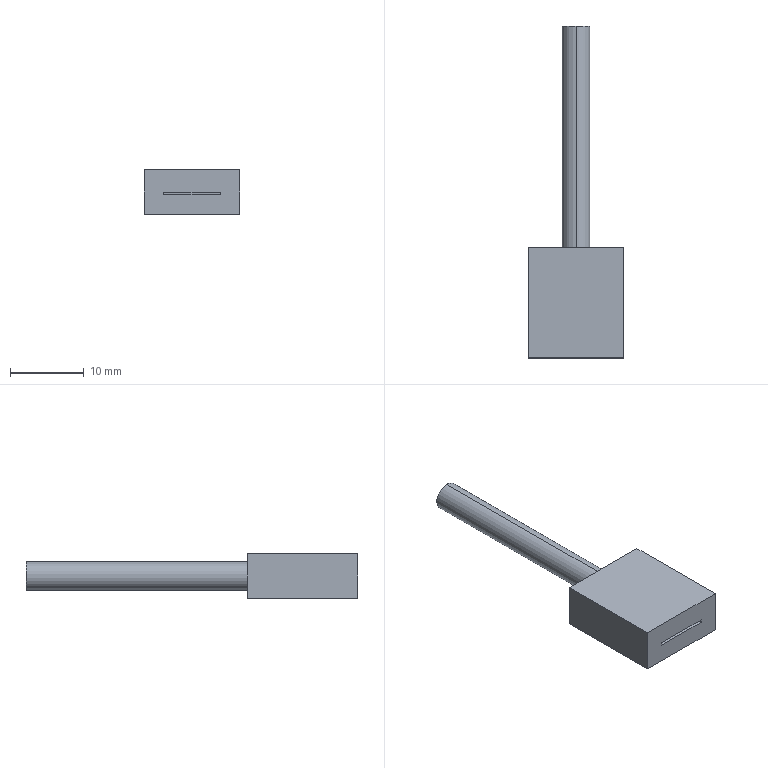Part | STEP file | 0244_012_FPCN14H | 1 solid | 14 faces | box 13 x 45 x 6 mm | volume 1495 mm3 | plane 12 | cylinder 2 | commonest cylinder face diameters 3.8 x2
STEP:
#1=CARTESIAN_POINT('',(0.,0.,0.));
#2=DIRECTION('',(0.,0.,1.));
#3=DIRECTION('',(1.,0.,0.));
#4=AXIS2_PLACEMENT_3D('',#1,#2,#3);
#5=CARTESIAN_POINT('',(0.,45.,-4.9));
#6=VERTEX_POINT('',#5);
#7=CARTESIAN_POINT('',(0.,45.,-1.1));
#8=VERTEX_POINT('',#7);
#9=CARTESIAN_POINT('',(0.,45.,-3.));
#10=DIRECTION('',(0.,-1.,0.));
#11=DIRECTION('',(0.,0.,-1.));
#12=AXIS2_PLACEMENT_3D('',#9,#10,#11);
#13=CIRCLE('',#12,1.9);
#14=CARTESIAN_POINT('',(0.,45.,-3.));
#15=DIRECTION('',(0.,-1.,0.));
#16=DIRECTION('',(0.,0.,-1.));
#17=AXIS2_PLACEMENT_3D('',#14,#15,#16);
#18=CYLINDRICAL_SURFACE('',#17,1.9);
#19=CARTESIAN_POINT('',(0.,0.));
#20=DIRECTION('',(1.,0.));
#21=VECTOR('',#20,1.);
#22=LINE('',#19,#21);
#23=(GEOMETRIC_REPRESENTATION_CONTEXT(2)PARAMETRIC_REPRESENTATION_CONTEXT()REPRESENTATION_CONTEXT('',''));
#24=DEFINITIONAL_REPRESENTATION('',(#22),#23);
#25=PCURVE('',#18,#24);
#26=CARTESIAN_POINT('',(0.,45.,-3.));
#27=DIRECTION('',(0.,1.,0.));
#28=DIRECTION('',(0.,0.,1.));
#29=AXIS2_PLACEMENT_3D('',#26,#27,#28);
#30=PLANE('',#29);
#31=CARTESIAN_POINT('',(-1.9,0.));
#32=CARTESIAN_POINT('',(-1.9,3.291));
#33=CARTESIAN_POINT('',(0.95,1.645));
#34=CARTESIAN_POINT('',(3.8,0.));
#35=CARTESIAN_POINT('',(0.95,-1.645));
#36=CARTESIAN_POINT('',(-1.9,-3.291));
#37=CARTESIAN_POINT('',(-1.9,0.));
#38=(BOUNDED_CURVE()B_SPLINE_CURVE(2,(#31,#32,#33,#34,#35,#36,#37),.UNSPECIFIED.,.T.,.F.)B_SPLINE_CURVE_WITH_KNOTS((1,2,2,2,2,1),(-2.094,0.,2.094,4.189,6.283,8.378),.UNSPECIFIED.)CURVE()GEOMETRIC_REPRESENTATION_ITEM()RATIONAL_B_SPLINE_CURVE((1.,0.5,1.,0.5,1.,0.5,1.))REPRESENTATION_ITEM(''));
#39=(GEOMETRIC_REPRESENTATION_CONTEXT(2)PARAMETRIC_REPRESENTATION_CONTEXT()REPRESENTATION_CONTEXT('',''));
#40=DEFINITIONAL_REPRESENTATION('',(#38),#39);
#41=PCURVE('',#30,#40);
#42=SURFACE_CURVE('',#13,(#25,#41),.PCURVE_S1.);
#43=EDGE_CURVE('',#6,#8,#42,.T.);
#44=ORIENTED_EDGE('',*,*,#43,.T.);
#45=CARTESIAN_POINT('',(0.,15.,-1.1));
#46=VERTEX_POINT('',#45);
#47=CARTESIAN_POINT('',(0.,45.,-1.1));
#48=DIRECTION('',(0.,-1.,0.));
#49=VECTOR('',#48,1.);
#50=LINE('',#47,#49);
#51=CARTESIAN_POINT('',(3.142,0.));
#52=DIRECTION('',(0.,1.));
#53=VECTOR('',#52,1.);
#54=LINE('',#51,#53);
#55=(GEOMETRIC_REPRESENTATION_CONTEXT(2)PARAMETRIC_REPRESENTATION_CONTEXT()REPRESENTATION_CONTEXT('',''));
#56=DEFINITIONAL_REPRESENTATION('',(#54),#55);
#57=PCURVE('',#18,#56);
#58=CARTESIAN_POINT('',(0.,45.,-3.));
#59=DIRECTION('',(0.,-1.,0.));
#60=DIRECTION('',(0.,0.,-1.));
#61=AXIS2_PLACEMENT_3D('',#58,#59,#60);
#62=CYLINDRICAL_SURFACE('',#61,1.9);
#63=CARTESIAN_POINT('',(3.142,0.));
#64=DIRECTION('',(0.,1.));
#65=VECTOR('',#64,1.);
#66=LINE('',#63,#65);
#67=(GEOMETRIC_REPRESENTATION_CONTEXT(2)PARAMETRIC_REPRESENTATION_CONTEXT()REPRESENTATION_CONTEXT('',''));
#68=DEFINITIONAL_REPRESENTATION('',(#66),#67);
#69=PCURVE('',#62,#68);
#70=SURFACE_CURVE('',#50,(#57,#69),.PCURVE_S1.);
#71=EDGE_CURVE('',#8,#46,#70,.T.);
#72=ORIENTED_EDGE('',*,*,#71,.T.);
#73=CARTESIAN_POINT('',(0.,15.,-4.9));
#74=VERTEX_POINT('',#73);
#75=CARTESIAN_POINT('',(0.,15.,-3.));
#76=DIRECTION('',(0.,1.,0.));
#77=DIRECTION('',(0.,0.,-1.));
#78=AXIS2_PLACEMENT_3D('',#75,#76,#77);
#79=CIRCLE('',#78,1.9);
#80=CARTESIAN_POINT('',(6.283,30.));
#81=DIRECTION('',(-1.,0.));
#82=VECTOR('',#81,1.);
#83=LINE('',#80,#82);
#84=(GEOMETRIC_REPRESENTATION_CONTEXT(2)PARAMETRIC_REPRESENTATION_CONTEXT()REPRESENTATION_CONTEXT('',''));
#85=DEFINITIONAL_REPRESENTATION('',(#83),#84);
#86=PCURVE('',#18,#85);
#87=CARTESIAN_POINT('',(6.5,15.,0.));
#88=DIRECTION('',(0.,-1.,0.));
#89=DIRECTION('',(0.,0.,-1.));
#90=AXIS2_PLACEMENT_3D('',#87,#88,#89);
#91=PLANE('',#90);
#92=CARTESIAN_POINT('',(4.9,-6.5));
#93=CARTESIAN_POINT('',(4.9,-9.791));
#94=CARTESIAN_POINT('',(2.05,-8.145));
#95=CARTESIAN_POINT('',(-0.8,-6.5));
#96=CARTESIAN_POINT('',(2.05,-4.855));
#97=CARTESIAN_POINT('',(4.9,-3.209));
#98=CARTESIAN_POINT('',(4.9,-6.5));
#99=(BOUNDED_CURVE()B_SPLINE_CURVE(2,(#92,#93,#94,#95,#96,#97,#98),.UNSPECIFIED.,.T.,.F.)B_SPLINE_CURVE_WITH_KNOTS((1,2,2,2,2,1),(-2.094,0.,2.094,4.189,6.283,8.378),.UNSPECIFIED.)CURVE()GEOMETRIC_REPRESENTATION_ITEM()RATIONAL_B_SPLINE_CURVE((1.,0.5,1.,0.5,1.,0.5,1.))REPRESENTATION_ITEM(''));
#100=(GEOMETRIC_REPRESENTATION_CONTEXT(2)PARAMETRIC_REPRESENTATION_CONTEXT()REPRESENTATION_CONTEXT('',''));
#101=DEFINITIONAL_REPRESENTATION('',(#99),#100);
#102=PCURVE('',#91,#101);
#103=SURFACE_CURVE('',#79,(#86,#102),.PCURVE_S1.);
#104=EDGE_CURVE('',#46,#74,#103,.T.);
#105=ORIENTED_EDGE('',*,*,#104,.T.);
#106=CARTESIAN_POINT('',(0.,45.,-4.9));
#107=DIRECTION('',(0.,-1.,0.));
#108=VECTOR('',#107,1.);
#109=LINE('',#106,#108);
#110=CARTESIAN_POINT('',(0.,0.));
#111=DIRECTION('',(0.,1.));
#112=VECTOR('',#111,1.);
#113=LINE('',#110,#112);
#114=(GEOMETRIC_REPRESENTATION_CONTEXT(2)PARAMETRIC_REPRESENTATION_CONTEXT()REPRESENTATION_CONTEXT('',''));
#115=DEFINITIONAL_REPRESENTATION('',(#113),#114);
#116=PCURVE('',#18,#115);
#117=CARTESIAN_POINT('',(6.283,0.));
#118=DIRECTION('',(0.,1.));
#119=VECTOR('',#118,1.);
#120=LINE('',#117,#119);
#121=(GEOMETRIC_REPRESENTATION_CONTEXT(2)PARAMETRIC_REPRESENTATION_CONTEXT()REPRESENTATION_CONTEXT('',''));
#122=DEFINITIONAL_REPRESENTATION('',(#120),#121);
#123=PCURVE('',#62,#122);
#124=SURFACE_CURVE('',#109,(#116,#123),.PCURVE_S1.);
#125=EDGE_CURVE('',#6,#74,#124,.T.);
#126=ORIENTED_EDGE('',*,*,#125,.F.);
#127=EDGE_LOOP('',(#44,#72,#105,#126));
#128=FACE_BOUND('',#127,.T.);
#129=ADVANCED_FACE('',(#128),#18,.T.);
#130=CARTESIAN_POINT('',(6.5,0.,0.));
#131=VERTEX_POINT('',#130);
#132=CARTESIAN_POINT('',(-6.5,0.,0.));
#133=VERTEX_POINT('',#132);
#134=CARTESIAN_POINT('',(6.5,0.,0.));
#135=DIRECTION('',(-1.,0.,0.));
#136=VECTOR('',#135,1.);
#137=LINE('',#134,#136);
#138=CARTESIAN_POINT('',(6.5,0.,0.));
#139=DIRECTION('',(0.,0.,-1.));
#140=DIRECTION('',(-1.,0.,0.));
#141=AXIS2_PLACEMENT_3D('',#138,#139,#140);
#142=PLANE('',#141);
#143=CARTESIAN_POINT('',(0.,0.));
#144=DIRECTION('',(1.,0.));
#145=VECTOR('',#144,1.);
#146=LINE('',#143,#145);
#147=(GEOMETRIC_REPRESENTATION_CONTEXT(2)PARAMETRIC_REPRESENTATION_CONTEXT()REPRESENTATION_CONTEXT('',''));
#148=DEFINITIONAL_REPRESENTATION('',(#146),#147);
#149=PCURVE('',#142,#148);
#150=CARTESIAN_POINT('',(6.5,0.,0.));
#151=DIRECTION('',(0.,1.,0.));
#152=DIRECTION('',(0.,0.,1.));
#153=AXIS2_PLACEMENT_3D('',#150,#151,#152);
#154=PLANE('',#153);
#155=CARTESIAN_POINT('',(0.,0.));
#156=DIRECTION('',(0.,-1.));
#157=VECTOR('',#156,1.);
#158=LINE('',#155,#157);
#159=(GEOMETRIC_REPRESENTATION_CONTEXT(2)PARAMETRIC_REPRESENTATION_CONTEXT()REPRESENTATION_CONTEXT('',''));
#160=DEFINITIONAL_REPRESENTATION('',(#158),#159);
#161=PCURVE('',#154,#160);
#162=SURFACE_CURVE('',#137,(#149,#161),.PCURVE_S1.);
#163=EDGE_CURVE('',#131,#133,#162,.T.);
#164=ORIENTED_EDGE('',*,*,#163,.F.);
#165=CARTESIAN_POINT('',(6.5,15.,0.));
#166=VERTEX_POINT('',#165);
#167=CARTESIAN_POINT('',(6.5,0.,0.));
#168=DIRECTION('',(0.,-1.,0.));
#169=VECTOR('',#168,1.);
#170=LINE('',#167,#169);
#171=CARTESIAN_POINT('',(0.,0.));
#172=DIRECTION('',(0.,-1.));
#173=VECTOR('',#172,1.);
#174=LINE('',#171,#173);
#175=(GEOMETRIC_REPRESENTATION_CONTEXT(2)PARAMETRIC_REPRESENTATION_CONTEXT()REPRESENTATION_CONTEXT('',''));
#176=DEFINITIONAL_REPRESENTATION('',(#174),#175);
#177=PCURVE('',#142,#176);
#178=CARTESIAN_POINT('',(6.5,15.,0.));
#179=DIRECTION('',(-1.,0.,0.));
#180=DIRECTION('',(0.,0.,1.));
#181=AXIS2_PLACEMENT_3D('',#178,#179,#180);
#182=PLANE('',#181);
#183=CARTESIAN_POINT('',(0.,-15.));
#184=DIRECTION('',(0.,-1.));
#185=VECTOR('',#184,1.);
#186=LINE('',#183,#185);
#187=(GEOMETRIC_REPRESENTATION_CONTEXT(2)PARAMETRIC_REPRESENTATION_CONTEXT()REPRESENTATION_CONTEXT('',''));
#188=DEFINITIONAL_REPRESENTATION('',(#186),#187);
#189=PCURVE('',#182,#188);
#190=SURFACE_CURVE('',#170,(#177,#189),.PCURVE_S1.);
#191=EDGE_CURVE('',#166,#131,#190,.T.);
#192=ORIENTED_EDGE('',*,*,#191,.F.);
#193=CARTESIAN_POINT('',(-6.5,15.,0.));
#194=VERTEX_POINT('',#193);
#195=CARTESIAN_POINT('',(6.5,15.,0.));
#196=DIRECTION('',(1.,0.,0.));
#197=VECTOR('',#196,1.);
#198=LINE('',#195,#197);
#199=CARTESIAN_POINT('',(0.,15.));
#200=DIRECTION('',(-1.,0.));
#201=VECTOR('',#200,1.);
#202=LINE('',#199,#201);
#203=(GEOMETRIC_REPRESENTATION_CONTEXT(2)PARAMETRIC_REPRESENTATION_CONTEXT()REPRESENTATION_CONTEXT('',''));
#204=DEFINITIONAL_REPRESENTATION('',(#202),#203);
#205=PCURVE('',#142,#204);
#206=CARTESIAN_POINT('',(0.,0.));
#207=DIRECTION('',(0.,1.));
#208=VECTOR('',#207,1.);
#209=LINE('',#206,#208);
#210=(GEOMETRIC_REPRESENTATION_CONTEXT(2)PARAMETRIC_REPRESENTATION_CONTEXT()REPRESENTATION_CONTEXT('',''));
#211=DEFINITIONAL_REPRESENTATION('',(#209),#210);
#212=PCURVE('',#91,#211);
#213=SURFACE_CURVE('',#198,(#205,#212),.PCURVE_S1.);
#214=EDGE_CURVE('',#194,#166,#213,.T.);
#215=ORIENTED_EDGE('',*,*,#214,.F.);
#216=CARTESIAN_POINT('',(-6.5,0.,0.));
#217=DIRECTION('',(0.,1.,0.));
#218=VECTOR('',#217,1.);
#219=LINE('',#216,#218);
#220=CARTESIAN_POINT('',(13.,0.));
#221=DIRECTION('',(0.,1.));
#222=VECTOR('',#221,1.);
#223=LINE('',#220,#222);
#224=(GEOMETRIC_REPRESENTATION_CONTEXT(2)PARAMETRIC_REPRESENTATION_CONTEXT()REPRESENTATION_CONTEXT('',''));
#225=DEFINITIONAL_REPRESENTATION('',(#223),#224);
#226=PCURVE('',#142,#225);
#227=CARTESIAN_POINT('',(-6.5,15.,0.));
#228=DIRECTION('',(-1.,0.,0.));
#229=DIRECTION('',(0.,0.,1.));
#230=AXIS2_PLACEMENT_3D('',#227,#228,#229);
#231=PLANE('',#230);
#232=CARTESIAN_POINT('',(0.,-15.));
#233=DIRECTION('',(0.,1.));
#234=VECTOR('',#233,1.);
#235=LINE('',#232,#234);
#236=(GEOMETRIC_REPRESENTATION_CONTEXT(2)PARAMETRIC_REPRESENTATION_CONTEXT()REPRESENTATION_CONTEXT('',''));
#237=DEFINITIONAL_REPRESENTATION('',(#235),#236);
#238=PCURVE('',#231,#237);
#239=SURFACE_CURVE('',#219,(#226,#238),.PCURVE_S1.);
#240=EDGE_CURVE('',#133,#194,#239,.T.);
#241=ORIENTED_EDGE('',*,*,#240,.F.);
#242=EDGE_LOOP('',(#164,#192,#215,#241));
#243=FACE_BOUND('',#242,.T.);
#244=ADVANCED_FACE('',(#243),#142,.F.);
#245=CARTESIAN_POINT('',(-6.5,15.,-6.));
#246=VERTEX_POINT('',#245);
#247=CARTESIAN_POINT('',(-6.5,0.,-6.));
#248=VERTEX_POINT('',#247);
#249=CARTESIAN_POINT('',(-6.5,15.,-6.));
#250=DIRECTION('',(0.,-1.,0.));
#251=VECTOR('',#250,1.);
#252=LINE('',#249,#251);
#253=CARTESIAN_POINT('',(-6.,0.));
#254=DIRECTION('',(0.,-1.));
#255=VECTOR('',#254,1.);
#256=LINE('',#253,#255);
#257=(GEOMETRIC_REPRESENTATION_CONTEXT(2)PARAMETRIC_REPRESENTATION_CONTEXT()REPRESENTATION_CONTEXT('',''));
#258=DEFINITIONAL_REPRESENTATION('',(#256),#257);
#259=PCURVE('',#231,#258);
#260=CARTESIAN_POINT('',(6.5,0.,-6.));
#261=DIRECTION('',(0.,0.,1.));
#262=DIRECTION('',(1.,0.,0.));
#263=AXIS2_PLACEMENT_3D('',#260,#261,#262);
#264=PLANE('',#263);
#265=CARTESIAN_POINT('',(-13.,15.));
#266=DIRECTION('',(0.,-1.));
#267=VECTOR('',#266,1.);
#268=LINE('',#265,#267);
#269=(GEOMETRIC_REPRESENTATION_CONTEXT(2)PARAMETRIC_REPRESENTATION_CONTEXT()REPRESENTATION_CONTEXT('',''));
#270=DEFINITIONAL_REPRESENTATION('',(#268),#269);
#271=PCURVE('',#264,#270);
#272=SURFACE_CURVE('',#252,(#259,#271),.PCURVE_S1.);
#273=EDGE_CURVE('',#246,#248,#272,.T.);
#274=ORIENTED_EDGE('',*,*,#273,.T.);
#275=CARTESIAN_POINT('',(-6.5,0.,0.));
#276=DIRECTION('',(0.,0.,1.));
#277=VECTOR('',#276,1.);
#278=LINE('',#275,#277);
#279=CARTESIAN_POINT('',(0.,-15.));
#280=DIRECTION('',(1.,0.));
#281=VECTOR('',#280,1.);
#282=LINE('',#279,#281);
#283=(GEOMETRIC_REPRESENTATION_CONTEXT(2)PARAMETRIC_REPRESENTATION_CONTEXT()REPRESENTATION_CONTEXT('',''));
#284=DEFINITIONAL_REPRESENTATION('',(#282),#283);
#285=PCURVE('',#231,#284);
#286=CARTESIAN_POINT('',(0.,-13.));
#287=DIRECTION('',(1.,0.));
#288=VECTOR('',#287,1.);
#289=LINE('',#286,#288);
#290=(GEOMETRIC_REPRESENTATION_CONTEXT(2)PARAMETRIC_REPRESENTATION_CONTEXT()REPRESENTATION_CONTEXT('',''));
#291=DEFINITIONAL_REPRESENTATION('',(#289),#290);
#292=PCURVE('',#154,#291);
#293=SURFACE_CURVE('',#278,(#285,#292),.PCURVE_S1.);
#294=EDGE_CURVE('',#248,#133,#293,.T.);
#295=ORIENTED_EDGE('',*,*,#294,.T.);
#296=ORIENTED_EDGE('',*,*,#240,.T.);
#297=CARTESIAN_POINT('',(-6.5,15.,0.));
#298=DIRECTION('',(0.,0.,-1.));
#299=VECTOR('',#298,1.);
#300=LINE('',#297,#299);
#301=CARTESIAN_POINT('',(0.,0.));
#302=DIRECTION('',(-1.,0.));
#303=VECTOR('',#302,1.);
#304=LINE('',#301,#303);
#305=(GEOMETRIC_REPRESENTATION_CONTEXT(2)PARAMETRIC_REPRESENTATION_CONTEXT()REPRESENTATION_CONTEXT('',''));
#306=DEFINITIONAL_REPRESENTATION('',(#304),#305);
#307=PCURVE('',#231,#306);
#308=CARTESIAN_POINT('',(0.,-13.));
#309=DIRECTION('',(1.,0.));
#310=VECTOR('',#309,1.);
#311=LINE('',#308,#310);
#312=(GEOMETRIC_REPRESENTATION_CONTEXT(2)PARAMETRIC_REPRESENTATION_CONTEXT()REPRESENTATION_CONTEXT('',''));
#313=DEFINITIONAL_REPRESENTATION('',(#311),#312);
#314=PCURVE('',#91,#313);
#315=SURFACE_CURVE('',#300,(#307,#314),.PCURVE_S1.);
#316=EDGE_CURVE('',#194,#246,#315,.T.);
#317=ORIENTED_EDGE('',*,*,#316,.T.);
#318=EDGE_LOOP('',(#274,#295,#296,#317));
#319=FACE_BOUND('',#318,.T.);
#320=ADVANCED_FACE('',(#319),#231,.T.);
#321=CARTESIAN_POINT('',(6.5,0.,-6.));
#322=VERTEX_POINT('',#321);
#323=CARTESIAN_POINT('',(6.5,0.,-6.));
#324=DIRECTION('',(-1.,0.,0.));
#325=VECTOR('',#324,1.);
#326=LINE('',#323,#325);
#327=CARTESIAN_POINT('',(-6.,0.));
#328=DIRECTION('',(0.,-1.));
#329=VECTOR('',#328,1.);
#330=LINE('',#327,#329);
#331=(GEOMETRIC_REPRESENTATION_CONTEXT(2)PARAMETRIC_REPRESENTATION_CONTEXT()REPRESENTATION_CONTEXT('',''));
#332=DEFINITIONAL_REPRESENTATION('',(#330),#331);
#333=PCURVE('',#154,#332);
#334=CARTESIAN_POINT('',(0.,0.));
#335=DIRECTION('',(-1.,0.));
#336=VECTOR('',#335,1.);
#337=LINE('',#334,#336);
#338=(GEOMETRIC_REPRESENTATION_CONTEXT(2)PARAMETRIC_REPRESENTATION_CONTEXT()REPRESENTATION_CONTEXT('',''));
#339=DEFINITIONAL_REPRESENTATION('',(#337),#338);
#340=PCURVE('',#264,#339);
#341=SURFACE_CURVE('',#326,(#333,#340),.PCURVE_S1.);
#342=EDGE_CURVE('',#322,#248,#341,.T.);
#343=ORIENTED_EDGE('',*,*,#342,.F.);
#344=CARTESIAN_POINT('',(6.5,0.,0.));
#345=DIRECTION('',(0.,0.,-1.));
#346=VECTOR('',#345,1.);
#347=LINE('',#344,#346);
#348=CARTESIAN_POINT('',(0.,0.));
#349=DIRECTION('',(-1.,0.));
#350=VECTOR('',#349,1.);
#351=LINE('',#348,#350);
#352=(GEOMETRIC_REPRESENTATION_CONTEXT(2)PARAMETRIC_REPRESENTATION_CONTEXT()REPRESENTATION_CONTEXT('',''));
#353=DEFINITIONAL_REPRESENTATION('',(#351),#352);
#354=PCURVE('',#154,#353);
#355=CARTESIAN_POINT('',(0.,-15.));
#356=DIRECTION('',(-1.,0.));
#357=VECTOR('',#356,1.);
#358=LINE('',#355,#357);
#359=(GEOMETRIC_REPRESENTATION_CONTEXT(2)PARAMETRIC_REPRESENTATION_CONTEXT()REPRESENTATION_CONTEXT('',''));
#360=DEFINITIONAL_REPRESENTATION('',(#358),#359);
#361=PCURVE('',#182,#360);
#362=SURFACE_CURVE('',#347,(#354,#361),.PCURVE_S1.);
#363=EDGE_CURVE('',#131,#322,#362,.T.);
#364=ORIENTED_EDGE('',*,*,#363,.F.);
#365=ORIENTED_EDGE('',*,*,#163,.T.);
#366=ORIENTED_EDGE('',*,*,#294,.F.);
#367=EDGE_LOOP('',(#343,#364,#365,#366));
#368=FACE_BOUND('',#367,.T.);
#369=CARTESIAN_POINT('',(-3.8,0.,-3.4));
#370=VERTEX_POINT('',#369);
#371=CARTESIAN_POINT('',(-3.8,0.,-3.));
#372=VERTEX_POINT('',#371);
#373=CARTESIAN_POINT('',(-3.8,0.,-3.));
#374=DIRECTION('',(0.,0.,1.));
#375=VECTOR('',#374,1.);
#376=LINE('',#373,#375);
#377=CARTESIAN_POINT('',(-3.,-10.3));
#378=DIRECTION('',(1.,0.));
#379=VECTOR('',#378,1.);
#380=LINE('',#377,#379);
#381=(GEOMETRIC_REPRESENTATION_CONTEXT(2)PARAMETRIC_REPRESENTATION_CONTEXT()REPRESENTATION_CONTEXT('',''));
#382=DEFINITIONAL_REPRESENTATION('',(#380),#381);
#383=PCURVE('',#154,#382);
#384=CARTESIAN_POINT('',(-3.8,5.,-3.));
#385=DIRECTION('',(-1.,0.,0.));
#386=DIRECTION('',(0.,0.,1.));
#387=AXIS2_PLACEMENT_3D('',#384,#385,#386);
#388=PLANE('',#387);
#389=CARTESIAN_POINT('',(0.,-5.));
#390=DIRECTION('',(1.,0.));
#391=VECTOR('',#390,1.);
#392=LINE('',#389,#391);
#393=(GEOMETRIC_REPRESENTATION_CONTEXT(2)PARAMETRIC_REPRESENTATION_CONTEXT()REPRESENTATION_CONTEXT('',''));
#394=DEFINITIONAL_REPRESENTATION('',(#392),#393);
#395=PCURVE('',#388,#394);
#396=SURFACE_CURVE('',#376,(#383,#395),.PCURVE_S1.);
#397=EDGE_CURVE('',#370,#372,#396,.T.);
#398=ORIENTED_EDGE('',*,*,#397,.T.);
#399=CARTESIAN_POINT('',(3.8,0.,-3.));
#400=VERTEX_POINT('',#399);
#401=CARTESIAN_POINT('',(6.5,0.,-3.));
#402=DIRECTION('',(-1.,0.,0.));
#403=VECTOR('',#402,1.);
#404=LINE('',#401,#403);
#405=CARTESIAN_POINT('',(-3.,0.));
#406=DIRECTION('',(0.,-1.));
#407=VECTOR('',#406,1.);
#408=LINE('',#405,#407);
#409=(GEOMETRIC_REPRESENTATION_CONTEXT(2)PARAMETRIC_REPRESENTATION_CONTEXT()REPRESENTATION_CONTEXT('',''));
#410=DEFINITIONAL_REPRESENTATION('',(#408),#409);
#411=PCURVE('',#154,#410);
#412=CARTESIAN_POINT('',(-3.8,5.,-3.));
#413=DIRECTION('',(0.,0.,1.));
#414=DIRECTION('',(1.,0.,0.));
#415=AXIS2_PLACEMENT_3D('',#412,#413,#414);
#416=PLANE('',#415);
#417=CARTESIAN_POINT('',(10.3,-5.));
#418=DIRECTION('',(-1.,0.));
#419=VECTOR('',#418,1.);
#420=LINE('',#417,#419);
#421=(GEOMETRIC_REPRESENTATION_CONTEXT(2)PARAMETRIC_REPRESENTATION_CONTEXT()REPRESENTATION_CONTEXT('',''));
#422=DEFINITIONAL_REPRESENTATION('',(#420),#421);
#423=PCURVE('',#416,#422);
#424=SURFACE_CURVE('',#404,(#411,#423),.PCURVE_S1.);
#425=EDGE_CURVE('',#400,#372,#424,.T.);
#426=ORIENTED_EDGE('',*,*,#425,.F.);
#427=CARTESIAN_POINT('',(3.8,0.,-3.4));
#428=VERTEX_POINT('',#427);
#429=CARTESIAN_POINT('',(3.8,0.,-3.));
#430=DIRECTION('',(0.,0.,-1.));
#431=VECTOR('',#430,1.);
#432=LINE('',#429,#431);
#433=CARTESIAN_POINT('',(-3.,-2.7));
#434=DIRECTION('',(-1.,0.));
#435=VECTOR('',#434,1.);
#436=LINE('',#433,#435);
#437=(GEOMETRIC_REPRESENTATION_CONTEXT(2)PARAMETRIC_REPRESENTATION_CONTEXT()REPRESENTATION_CONTEXT('',''));
#438=DEFINITIONAL_REPRESENTATION('',(#436),#437);
#439=PCURVE('',#154,#438);
#440=CARTESIAN_POINT('',(3.8,5.,-3.));
#441=DIRECTION('',(1.,0.,0.));
#442=DIRECTION('',(0.,0.,-1.));
#443=AXIS2_PLACEMENT_3D('',#440,#441,#442);
#444=PLANE('',#443);
#445=CARTESIAN_POINT('',(0.,-5.));
#446=DIRECTION('',(1.,0.));
#447=VECTOR('',#446,1.);
#448=LINE('',#445,#447);
#449=(GEOMETRIC_REPRESENTATION_CONTEXT(2)PARAMETRIC_REPRESENTATION_CONTEXT()REPRESENTATION_CONTEXT('',''));
#450=DEFINITIONAL_REPRESENTATION('',(#448),#449);
#451=PCURVE('',#444,#450);
#452=SURFACE_CURVE('',#432,(#439,#451),.PCURVE_S1.);
#453=EDGE_CURVE('',#400,#428,#452,.T.);
#454=ORIENTED_EDGE('',*,*,#453,.T.);
#455=CARTESIAN_POINT('',(6.5,0.,-3.4));
#456=DIRECTION('',(1.,0.,0.));
#457=VECTOR('',#456,1.);
#458=LINE('',#455,#457);
#459=CARTESIAN_POINT('',(-3.4,0.));
#460=DIRECTION('',(0.,1.));
#461=VECTOR('',#460,1.);
#462=LINE('',#459,#461);
#463=(GEOMETRIC_REPRESENTATION_CONTEXT(2)PARAMETRIC_REPRESENTATION_CONTEXT()REPRESENTATION_CONTEXT('',''));
#464=DEFINITIONAL_REPRESENTATION('',(#462),#463);
#465=PCURVE('',#154,#464);
#466=CARTESIAN_POINT('',(-3.8,5.,-3.4));
#467=DIRECTION('',(0.,0.,-1.));
#468=DIRECTION('',(-1.,0.,0.));
#469=AXIS2_PLACEMENT_3D('',#466,#467,#468);
#470=PLANE('',#469);
#471=CARTESIAN_POINT('',(-10.3,-5.));
#472=DIRECTION('',(-1.,0.));
#473=VECTOR('',#472,1.);
#474=LINE('',#471,#473);
#475=(GEOMETRIC_REPRESENTATION_CONTEXT(2)PARAMETRIC_REPRESENTATION_CONTEXT()REPRESENTATION_CONTEXT('',''));
#476=DEFINITIONAL_REPRESENTATION('',(#474),#475);
#477=PCURVE('',#470,#476);
#478=SURFACE_CURVE('',#458,(#465,#477),.PCURVE_S1.);
#479=EDGE_CURVE('',#370,#428,#478,.T.);
#480=ORIENTED_EDGE('',*,*,#479,.F.);
#481=EDGE_LOOP('',(#398,#426,#454,#480));
#482=FACE_BOUND('',#481,.T.);
#483=ADVANCED_FACE('',(#368,#482),#154,.F.);
#484=ORIENTED_EDGE('',*,*,#363,.T.);
#485=CARTESIAN_POINT('',(6.5,15.,-6.));
#486=VERTEX_POINT('',#485);
#487=CARTESIAN_POINT('',(6.5,15.,-6.));
#488=DIRECTION('',(0.,-1.,0.));
#489=VECTOR('',#488,1.);
#490=LINE('',#487,#489);
#491=CARTESIAN_POINT('',(-6.,0.));
#492=DIRECTION('',(0.,-1.));
#493=VECTOR('',#492,1.);
#494=LINE('',#491,#493);
#495=(GEOMETRIC_REPRESENTATION_CONTEXT(2)PARAMETRIC_REPRESENTATION_CONTEXT()REPRESENTATION_CONTEXT('',''));
#496=DEFINITIONAL_REPRESENTATION('',(#494),#495);
#497=PCURVE('',#182,#496);
#498=CARTESIAN_POINT('',(0.,15.));
#499=DIRECTION('',(0.,-1.));
#500=VECTOR('',#499,1.);
#501=LINE('',#498,#500);
#502=(GEOMETRIC_REPRESENTATION_CONTEXT(2)PARAMETRIC_REPRESENTATION_CONTEXT()REPRESENTATION_CONTEXT('',''));
#503=DEFINITIONAL_REPRESENTATION('',(#501),#502);
#504=PCURVE('',#264,#503);
#505=SURFACE_CURVE('',#490,(#497,#504),.PCURVE_S1.);
#506=EDGE_CURVE('',#486,#322,#505,.T.);
#507=ORIENTED_EDGE('',*,*,#506,.F.);
#508=CARTESIAN_POINT('',(6.5,15.,0.));
#509=DIRECTION('',(0.,0.,-1.));
#510=VECTOR('',#509,1.);
#511=LINE('',#508,#510);
#512=CARTESIAN_POINT('',(0.,0.));
#513=DIRECTION('',(-1.,0.));
#514=VECTOR('',#513,1.);
#515=LINE('',#512,#514);
#516=(GEOMETRIC_REPRESENTATION_CONTEXT(2)PARAMETRIC_REPRESENTATION_CONTEXT()REPRESENTATION_CONTEXT('',''));
#517=DEFINITIONAL_REPRESENTATION('',(#515),#516);
#518=PCURVE('',#182,#517);
#519=CARTESIAN_POINT('',(0.,0.));
#520=DIRECTION('',(1.,0.));
#521=VECTOR('',#520,1.);
#522=LINE('',#519,#521);
#523=(GEOMETRIC_REPRESENTATION_CONTEXT(2)PARAMETRIC_REPRESENTATION_CONTEXT()REPRESENTATION_CONTEXT('',''));
#524=DEFINITIONAL_REPRESENTATION('',(#522),#523);
#525=PCURVE('',#91,#524);
#526=SURFACE_CURVE('',#511,(#518,#525),.PCURVE_S1.);
#527=EDGE_CURVE('',#166,#486,#526,.T.);
#528=ORIENTED_EDGE('',*,*,#527,.F.);
#529=ORIENTED_EDGE('',*,*,#191,.T.);
#530=EDGE_LOOP('',(#484,#507,#528,#529));
#531=FACE_BOUND('',#530,.T.);
#532=ADVANCED_FACE('',(#531),#182,.F.);
#533=CARTESIAN_POINT('',(0.,15.,-3.));
#534=DIRECTION('',(0.,1.,0.));
#535=DIRECTION('',(0.,0.,-1.));
#536=AXIS2_PLACEMENT_3D('',#533,#534,#535);
#537=CIRCLE('',#536,1.9);
#538=CARTESIAN_POINT('',(4.9,-6.5));
#539=CARTESIAN_POINT('',(4.9,-9.791));
#540=CARTESIAN_POINT('',(2.05,-8.145));
#541=CARTESIAN_POINT('',(-0.8,-6.5));
#542=CARTESIAN_POINT('',(2.05,-4.855));
#543=CARTESIAN_POINT('',(4.9,-3.209));
#544=CARTESIAN_POINT('',(4.9,-6.5));
#545=(BOUNDED_CURVE()B_SPLINE_CURVE(2,(#538,#539,#540,#541,#542,#543,#544),.UNSPECIFIED.,.T.,.F.)B_SPLINE_CURVE_WITH_KNOTS((1,2,2,2,2,1),(-2.094,0.,2.094,4.189,6.283,8.378),.UNSPECIFIED.)CURVE()GEOMETRIC_REPRESENTATION_ITEM()RATIONAL_B_SPLINE_CURVE((1.,0.5,1.,0.5,1.,0.5,1.))REPRESENTATION_ITEM(''));
#546=(GEOMETRIC_REPRESENTATION_CONTEXT(2)PARAMETRIC_REPRESENTATION_CONTEXT()REPRESENTATION_CONTEXT('',''));
#547=DEFINITIONAL_REPRESENTATION('',(#545),#546);
#548=PCURVE('',#91,#547);
#549=CARTESIAN_POINT('',(6.283,30.));
#550=DIRECTION('',(-1.,0.));
#551=VECTOR('',#550,1.);
#552=LINE('',#549,#551);
#553=(GEOMETRIC_REPRESENTATION_CONTEXT(2)PARAMETRIC_REPRESENTATION_CONTEXT()REPRESENTATION_CONTEXT('',''));
#554=DEFINITIONAL_REPRESENTATION('',(#552),#553);
#555=PCURVE('',#62,#554);
#556=SURFACE_CURVE('',#537,(#548,#555),.PCURVE_S1.);
#557=EDGE_CURVE('',#74,#46,#556,.T.);
#558=ORIENTED_EDGE('',*,*,#557,.F.);
#559=ORIENTED_EDGE('',*,*,#104,.F.);
#560=EDGE_LOOP('',(#558,#559));
#561=FACE_BOUND('',#560,.T.);
#562=ORIENTED_EDGE('',*,*,#214,.T.);
#563=ORIENTED_EDGE('',*,*,#527,.T.);
#564=CARTESIAN_POINT('',(6.5,15.,-6.));
#565=DIRECTION('',(1.,0.,0.));
#566=VECTOR('',#565,1.);
#567=LINE('',#564,#566);
#568=CARTESIAN_POINT('',(6.,0.));
#569=DIRECTION('',(0.,1.));
#570=VECTOR('',#569,1.);
#571=LINE('',#568,#570);
#572=(GEOMETRIC_REPRESENTATION_CONTEXT(2)PARAMETRIC_REPRESENTATION_CONTEXT()REPRESENTATION_CONTEXT('',''));
#573=DEFINITIONAL_REPRESENTATION('',(#571),#572);
#574=PCURVE('',#91,#573);
#575=CARTESIAN_POINT('',(0.,15.));
#576=DIRECTION('',(1.,0.));
#577=VECTOR('',#576,1.);
#578=LINE('',#575,#577);
#579=(GEOMETRIC_REPRESENTATION_CONTEXT(2)PARAMETRIC_REPRESENTATION_CONTEXT()REPRESENTATION_CONTEXT('',''));
#580=DEFINITIONAL_REPRESENTATION('',(#578),#579);
#581=PCURVE('',#264,#580);
#582=SURFACE_CURVE('',#567,(#574,#581),.PCURVE_S1.);
#583=EDGE_CURVE('',#246,#486,#582,.T.);
#584=ORIENTED_EDGE('',*,*,#583,.F.);
#585=ORIENTED_EDGE('',*,*,#316,.F.);
#586=EDGE_LOOP('',(#562,#563,#584,#585));
#587=FACE_BOUND('',#586,.T.);
#588=ADVANCED_FACE('',(#561,#587),#91,.F.);
#589=ORIENTED_EDGE('',*,*,#583,.T.);
#590=ORIENTED_EDGE('',*,*,#506,.T.);
#591=ORIENTED_EDGE('',*,*,#342,.T.);
#592=ORIENTED_EDGE('',*,*,#273,.F.);
#593=EDGE_LOOP('',(#589,#590,#591,#592));
#594=FACE_BOUND('',#593,.T.);
#595=ADVANCED_FACE('',(#594),#264,.F.);
#596=CARTESIAN_POINT('',(3.8,5.,-3.4));
#597=VERTEX_POINT('',#596);
#598=CARTESIAN_POINT('',(3.8,5.,-3.4));
#599=DIRECTION('',(0.,-1.,0.));
#600=VECTOR('',#599,1.);
#601=LINE('',#598,#600);
#602=CARTESIAN_POINT('',(-7.6,0.));
#603=DIRECTION('',(0.,-1.));
#604=VECTOR('',#603,1.);
#605=LINE('',#602,#604);
#606=(GEOMETRIC_REPRESENTATION_CONTEXT(2)PARAMETRIC_REPRESENTATION_CONTEXT()REPRESENTATION_CONTEXT('',''));
#607=DEFINITIONAL_REPRESENTATION('',(#605),#606);
#608=PCURVE('',#470,#607);
#609=CARTESIAN_POINT('',(0.4,0.));
#610=DIRECTION('',(0.,-1.));
#611=VECTOR('',#610,1.);
#612=LINE('',#609,#611);
#613=(GEOMETRIC_REPRESENTATION_CONTEXT(2)PARAMETRIC_REPRESENTATION_CONTEXT()REPRESENTATION_CONTEXT('',''));
#614=DEFINITIONAL_REPRESENTATION('',(#612),#613);
#615=PCURVE('',#444,#614);
#616=SURFACE_CURVE('',#601,(#608,#615),.PCURVE_S1.);
#617=EDGE_CURVE('',#597,#428,#616,.T.);
#618=ORIENTED_EDGE('',*,*,#617,.F.);
#619=CARTESIAN_POINT('',(-3.8,5.,-3.4));
#620=VERTEX_POINT('',#619);
#621=CARTESIAN_POINT('',(-3.8,5.,-3.4));
#622=DIRECTION('',(1.,0.,0.));
#623=VECTOR('',#622,1.);
#624=LINE('',#621,#623);
#625=CARTESIAN_POINT('',(0.,0.));
#626=DIRECTION('',(-1.,0.));
#627=VECTOR('',#626,1.);
#628=LINE('',#625,#627);
#629=(GEOMETRIC_REPRESENTATION_CONTEXT(2)PARAMETRIC_REPRESENTATION_CONTEXT()REPRESENTATION_CONTEXT('',''));
#630=DEFINITIONAL_REPRESENTATION('',(#628),#629);
#631=PCURVE('',#470,#630);
#632=CARTESIAN_POINT('',(-3.8,5.,-3.4));
#633=DIRECTION('',(0.,-1.,0.));
#634=DIRECTION('',(0.,0.,-1.));
#635=AXIS2_PLACEMENT_3D('',#632,#633,#634);
#636=PLANE('',#635);
#637=CARTESIAN_POINT('',(0.,0.));
#638=DIRECTION('',(0.,1.));
#639=VECTOR('',#638,1.);
#640=LINE('',#637,#639);
#641=(GEOMETRIC_REPRESENTATION_CONTEXT(2)PARAMETRIC_REPRESENTATION_CONTEXT()REPRESENTATION_CONTEXT('',''));
#642=DEFINITIONAL_REPRESENTATION('',(#640),#641);
#643=PCURVE('',#636,#642);
#644=SURFACE_CURVE('',#624,(#631,#643),.PCURVE_S1.);
#645=EDGE_CURVE('',#620,#597,#644,.T.);
#646=ORIENTED_EDGE('',*,*,#645,.F.);
#647=CARTESIAN_POINT('',(-3.8,5.,-3.4));
#648=DIRECTION('',(0.,1.,0.));
#649=VECTOR('',#648,1.);
#650=LINE('',#647,#649);
#651=CARTESIAN_POINT('',(0.,0.));
#652=DIRECTION('',(0.,1.));
#653=VECTOR('',#652,1.);
#654=LINE('',#651,#653);
#655=(GEOMETRIC_REPRESENTATION_CONTEXT(2)PARAMETRIC_REPRESENTATION_CONTEXT()REPRESENTATION_CONTEXT('',''));
#656=DEFINITIONAL_REPRESENTATION('',(#654),#655);
#657=PCURVE('',#470,#656);
#658=CARTESIAN_POINT('',(-0.4,0.));
#659=DIRECTION('',(0.,1.));
#660=VECTOR('',#659,1.);
#661=LINE('',#658,#660);
#662=(GEOMETRIC_REPRESENTATION_CONTEXT(2)PARAMETRIC_REPRESENTATION_CONTEXT()REPRESENTATION_CONTEXT('',''));
#663=DEFINITIONAL_REPRESENTATION('',(#661),#662);
#664=PCURVE('',#388,#663);
#665=SURFACE_CURVE('',#650,(#657,#664),.PCURVE_S1.);
#666=EDGE_CURVE('',#370,#620,#665,.T.);
#667=ORIENTED_EDGE('',*,*,#666,.F.);
#668=ORIENTED_EDGE('',*,*,#479,.T.);
#669=EDGE_LOOP('',(#618,#646,#667,#668));
#670=FACE_BOUND('',#669,.T.);
#671=ADVANCED_FACE('',(#670),#470,.F.);
#672=CARTESIAN_POINT('',(-3.8,5.,-3.));
#673=VERTEX_POINT('',#672);
#674=CARTESIAN_POINT('',(-3.8,5.,-3.));
#675=DIRECTION('',(0.,-1.,0.));
#676=VECTOR('',#675,1.);
#677=LINE('',#674,#676);
#678=CARTESIAN_POINT('',(0.,0.));
#679=DIRECTION('',(0.,-1.));
#680=VECTOR('',#679,1.);
#681=LINE('',#678,#680);
#682=(GEOMETRIC_REPRESENTATION_CONTEXT(2)PARAMETRIC_REPRESENTATION_CONTEXT()REPRESENTATION_CONTEXT('',''));
#683=DEFINITIONAL_REPRESENTATION('',(#681),#682);
#684=PCURVE('',#416,#683);
#685=CARTESIAN_POINT('',(0.,0.));
#686=DIRECTION('',(0.,-1.));
#687=VECTOR('',#686,1.);
#688=LINE('',#685,#687);
#689=(GEOMETRIC_REPRESENTATION_CONTEXT(2)PARAMETRIC_REPRESENTATION_CONTEXT()REPRESENTATION_CONTEXT('',''));
#690=DEFINITIONAL_REPRESENTATION('',(#688),#689);
#691=PCURVE('',#388,#690);
#692=SURFACE_CURVE('',#677,(#684,#691),.PCURVE_S1.);
#693=EDGE_CURVE('',#673,#372,#692,.T.);
#694=ORIENTED_EDGE('',*,*,#693,.F.);
#695=CARTESIAN_POINT('',(3.8,5.,-3.));
#696=VERTEX_POINT('',#695);
#697=CARTESIAN_POINT('',(-3.8,5.,-3.));
#698=DIRECTION('',(-1.,0.,0.));
#699=VECTOR('',#698,1.);
#700=LINE('',#697,#699);
#701=CARTESIAN_POINT('',(0.,0.));
#702=DIRECTION('',(-1.,0.));
#703=VECTOR('',#702,1.);
#704=LINE('',#701,#703);
#705=(GEOMETRIC_REPRESENTATION_CONTEXT(2)PARAMETRIC_REPRESENTATION_CONTEXT()REPRESENTATION_CONTEXT('',''));
#706=DEFINITIONAL_REPRESENTATION('',(#704),#705);
#707=PCURVE('',#416,#706);
#708=CARTESIAN_POINT('',(-0.4,0.));
#709=DIRECTION('',(0.,-1.));
#710=VECTOR('',#709,1.);
#711=LINE('',#708,#710);
#712=(GEOMETRIC_REPRESENTATION_CONTEXT(2)PARAMETRIC_REPRESENTATION_CONTEXT()REPRESENTATION_CONTEXT('',''));
#713=DEFINITIONAL_REPRESENTATION('',(#711),#712);
#714=PCURVE('',#636,#713);
#715=SURFACE_CURVE('',#700,(#707,#714),.PCURVE_S1.);
#716=EDGE_CURVE('',#696,#673,#715,.T.);
#717=ORIENTED_EDGE('',*,*,#716,.F.);
#718=CARTESIAN_POINT('',(3.8,5.,-3.));
#719=DIRECTION('',(0.,1.,0.));
#720=VECTOR('',#719,1.);
#721=LINE('',#718,#720);
#722=CARTESIAN_POINT('',(7.6,0.));
#723=DIRECTION('',(0.,1.));
#724=VECTOR('',#723,1.);
#725=LINE('',#722,#724);
#726=(GEOMETRIC_REPRESENTATION_CONTEXT(2)PARAMETRIC_REPRESENTATION_CONTEXT()REPRESENTATION_CONTEXT('',''));
#727=DEFINITIONAL_REPRESENTATION('',(#725),#726);
#728=PCURVE('',#416,#727);
#729=CARTESIAN_POINT('',(0.,0.));
#730=DIRECTION('',(0.,1.));
#731=VECTOR('',#730,1.);
#732=LINE('',#729,#731);
#733=(GEOMETRIC_REPRESENTATION_CONTEXT(2)PARAMETRIC_REPRESENTATION_CONTEXT()REPRESENTATION_CONTEXT('',''));
#734=DEFINITIONAL_REPRESENTATION('',(#732),#733);
#735=PCURVE('',#444,#734);
#736=SURFACE_CURVE('',#721,(#728,#735),.PCURVE_S1.);
#737=EDGE_CURVE('',#400,#696,#736,.T.);
#738=ORIENTED_EDGE('',*,*,#737,.F.);
#739=ORIENTED_EDGE('',*,*,#425,.T.);
#740=EDGE_LOOP('',(#694,#717,#738,#739));
#741=FACE_BOUND('',#740,.T.);
#742=ADVANCED_FACE('',(#741),#416,.F.);
#743=ORIENTED_EDGE('',*,*,#71,.F.);
#744=CARTESIAN_POINT('',(0.,45.,-3.));
#745=DIRECTION('',(0.,-1.,0.));
#746=DIRECTION('',(0.,0.,-1.));
#747=AXIS2_PLACEMENT_3D('',#744,#745,#746);
#748=CIRCLE('',#747,1.9);
#749=CARTESIAN_POINT('',(0.,0.));
#750=DIRECTION('',(1.,0.));
#751=VECTOR('',#750,1.);
#752=LINE('',#749,#751);
#753=(GEOMETRIC_REPRESENTATION_CONTEXT(2)PARAMETRIC_REPRESENTATION_CONTEXT()REPRESENTATION_CONTEXT('',''));
#754=DEFINITIONAL_REPRESENTATION('',(#752),#753);
#755=PCURVE('',#62,#754);
#756=CARTESIAN_POINT('',(-1.9,0.));
#757=CARTESIAN_POINT('',(-1.9,3.291));
#758=CARTESIAN_POINT('',(0.95,1.645));
#759=CARTESIAN_POINT('',(3.8,0.));
#760=CARTESIAN_POINT('',(0.95,-1.645));
#761=CARTESIAN_POINT('',(-1.9,-3.291));
#762=CARTESIAN_POINT('',(-1.9,0.));
#763=(BOUNDED_CURVE()B_SPLINE_CURVE(2,(#756,#757,#758,#759,#760,#761,#762),.UNSPECIFIED.,.T.,.F.)B_SPLINE_CURVE_WITH_KNOTS((1,2,2,2,2,1),(-2.094,0.,2.094,4.189,6.283,8.378),.UNSPECIFIED.)CURVE()GEOMETRIC_REPRESENTATION_ITEM()RATIONAL_B_SPLINE_CURVE((1.,0.5,1.,0.5,1.,0.5,1.))REPRESENTATION_ITEM(''));
#764=(GEOMETRIC_REPRESENTATION_CONTEXT(2)PARAMETRIC_REPRESENTATION_CONTEXT()REPRESENTATION_CONTEXT('',''));
#765=DEFINITIONAL_REPRESENTATION('',(#763),#764);
#766=PCURVE('',#30,#765);
#767=SURFACE_CURVE('',#748,(#755,#766),.PCURVE_S1.);
#768=EDGE_CURVE('',#8,#6,#767,.T.);
#769=ORIENTED_EDGE('',*,*,#768,.T.);
#770=ORIENTED_EDGE('',*,*,#125,.T.);
#771=ORIENTED_EDGE('',*,*,#557,.T.);
#772=EDGE_LOOP('',(#743,#769,#770,#771));
#773=FACE_BOUND('',#772,.T.);
#774=ADVANCED_FACE('',(#773),#62,.T.);
#775=ORIENTED_EDGE('',*,*,#737,.T.);
#776=CARTESIAN_POINT('',(3.8,5.,-3.));
#777=DIRECTION('',(0.,0.,1.));
#778=VECTOR('',#777,1.);
#779=LINE('',#776,#778);
#780=CARTESIAN_POINT('',(0.,0.));
#781=DIRECTION('',(-1.,0.));
#782=VECTOR('',#781,1.);
#783=LINE('',#780,#782);
#784=(GEOMETRIC_REPRESENTATION_CONTEXT(2)PARAMETRIC_REPRESENTATION_CONTEXT()REPRESENTATION_CONTEXT('',''));
#785=DEFINITIONAL_REPRESENTATION('',(#783),#784);
#786=PCURVE('',#444,#785);
#787=CARTESIAN_POINT('',(-0.4,7.6));
#788=DIRECTION('',(-1.,0.));
#789=VECTOR('',#788,1.);
#790=LINE('',#787,#789);
#791=(GEOMETRIC_REPRESENTATION_CONTEXT(2)PARAMETRIC_REPRESENTATION_CONTEXT()REPRESENTATION_CONTEXT('',''));
#792=DEFINITIONAL_REPRESENTATION('',(#790),#791);
#793=PCURVE('',#636,#792);
#794=SURFACE_CURVE('',#779,(#786,#793),.PCURVE_S1.);
#795=EDGE_CURVE('',#597,#696,#794,.T.);
#796=ORIENTED_EDGE('',*,*,#795,.F.);
#797=ORIENTED_EDGE('',*,*,#617,.T.);
#798=ORIENTED_EDGE('',*,*,#453,.F.);
#799=EDGE_LOOP('',(#775,#796,#797,#798));
#800=FACE_BOUND('',#799,.T.);
#801=ADVANCED_FACE('',(#800),#444,.F.);
#802=ORIENTED_EDGE('',*,*,#795,.T.);
#803=ORIENTED_EDGE('',*,*,#716,.T.);
#804=CARTESIAN_POINT('',(-3.8,5.,-3.4));
#805=DIRECTION('',(0.,0.,-1.));
#806=VECTOR('',#805,1.);
#807=LINE('',#804,#806);
#808=CARTESIAN_POINT('',(0.,0.));
#809=DIRECTION('',(1.,0.));
#810=VECTOR('',#809,1.);
#811=LINE('',#808,#810);
#812=(GEOMETRIC_REPRESENTATION_CONTEXT(2)PARAMETRIC_REPRESENTATION_CONTEXT()REPRESENTATION_CONTEXT('',''));
#813=DEFINITIONAL_REPRESENTATION('',(#811),#812);
#814=PCURVE('',#636,#813);
#815=CARTESIAN_POINT('',(-0.4,0.));
#816=DIRECTION('',(-1.,0.));
#817=VECTOR('',#816,1.);
#818=LINE('',#815,#817);
#819=(GEOMETRIC_REPRESENTATION_CONTEXT(2)PARAMETRIC_REPRESENTATION_CONTEXT()REPRESENTATION_CONTEXT('',''));
#820=DEFINITIONAL_REPRESENTATION('',(#818),#819);
#821=PCURVE('',#388,#820);
#822=SURFACE_CURVE('',#807,(#814,#821),.PCURVE_S1.);
#823=EDGE_CURVE('',#673,#620,#822,.T.);
#824=ORIENTED_EDGE('',*,*,#823,.T.);
#825=ORIENTED_EDGE('',*,*,#645,.T.);
#826=EDGE_LOOP('',(#802,#803,#824,#825));
#827=FACE_BOUND('',#826,.T.);
#828=ADVANCED_FACE('',(#827),#636,.T.);
#829=ORIENTED_EDGE('',*,*,#666,.T.);
#830=ORIENTED_EDGE('',*,*,#823,.F.);
#831=ORIENTED_EDGE('',*,*,#693,.T.);
#832=ORIENTED_EDGE('',*,*,#397,.F.);
#833=EDGE_LOOP('',(#829,#830,#831,#832));
#834=FACE_BOUND('',#833,.T.);
#835=ADVANCED_FACE('',(#834),#388,.F.);
#836=ORIENTED_EDGE('',*,*,#43,.F.);
#837=ORIENTED_EDGE('',*,*,#768,.F.);
#838=EDGE_LOOP('',(#836,#837));
#839=FACE_BOUND('',#838,.T.);
#840=ADVANCED_FACE('',(#839),#30,.T.);
#841=CLOSED_SHELL('',(#129,#244,#320,#483,#532,#588,#595,#671,#742,#774,#801,#828,#835,#840));
#842=MANIFOLD_SOLID_BREP('',#841);
#843=(LENGTH_UNIT()NAMED_UNIT(*)SI_UNIT(.MILLI.,.METRE.));
#844=UNCERTAINTY_MEASURE_WITH_UNIT(LENGTH_MEASURE(0.0000001),#843,'','');
#845=(NAMED_UNIT(*)PLANE_ANGLE_UNIT()SI_UNIT($,.RADIAN.));
#846=(NAMED_UNIT(*)SI_UNIT($,.STERADIAN.)SOLID_ANGLE_UNIT());
#847=(GEOMETRIC_REPRESENTATION_CONTEXT(3)GLOBAL_UNCERTAINTY_ASSIGNED_CONTEXT((#844))GLOBAL_UNIT_ASSIGNED_CONTEXT((#843,#845,#846))REPRESENTATION_CONTEXT('',''));
#848=ADVANCED_BREP_SHAPE_REPRESENTATION('',(#4,#842),#847);